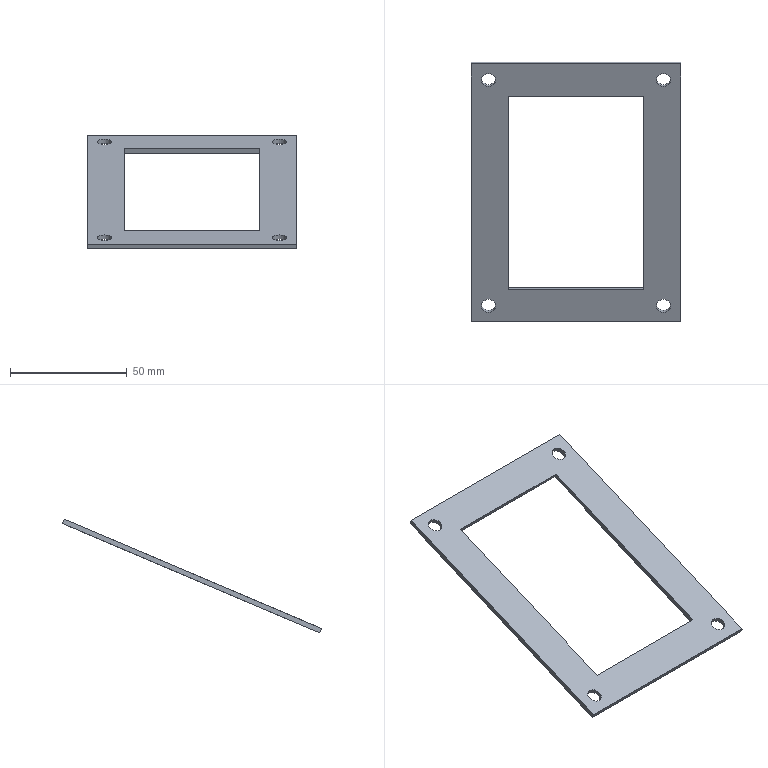Part | NX | features SIMPLE HOLE 56, DATUM_CSYS 27, HOLE PACKAGE 26, SKETCH 26, EXTRUDE 18, EXTRACT_FACE 16, EXTRACT_DATUM_AXIS 10, BLEND 8, CBORE_HOLE 7, EXTRACT_DATUM_PLANE 6, FSET 6, Instance Feature 5, Mirror Feature 5, DRAFT 4, EXTRACT_STRING 2, OFFSET_REGION 1 | 1 solid | 14 faces | box 90 x 111.242 x 48.729 mm | volume 10934 mm3 | plane 10 | cylinder 4 | commonest cylinder face diameters 6 x4
STEP:
#1=CARTESIAN_POINT('',(-45.,-37.433,105.427));
#2=VERTEX_POINT('',#1);
#3=CARTESIAN_POINT('',(-45.,73.028,152.315));
#4=VERTEX_POINT('',#3);
#5=CARTESIAN_POINT('',(-45.,73.028,152.315));
#6=DIRECTION('',(0.,0.9205,0.3907));
#7=VECTOR('',#6,1000.);
#8=LINE('',#5,#7);
#9=EDGE_CURVE('',#2,#4,#8,.T.);
#10=ORIENTED_EDGE('',*,*,#9,.F.);
#11=CARTESIAN_POINT('',(-45.,-38.214,107.268));
#12=VERTEX_POINT('',#11);
#13=CARTESIAN_POINT('',(-45.,17.27,-23.444));
#14=DIRECTION('',(0.,-0.3907,0.9205));
#15=VECTOR('',#14,1000.);
#16=LINE('',#13,#15);
#17=EDGE_CURVE('',#2,#12,#16,.T.);
#18=ORIENTED_EDGE('',*,*,#17,.T.);
#19=CARTESIAN_POINT('',(-45.,72.246,154.156));
#20=VERTEX_POINT('',#19);
#21=CARTESIAN_POINT('',(-45.,72.246,154.156));
#22=DIRECTION('',(0.,-0.9205,-0.3907));
#23=VECTOR('',#22,1000.);
#24=LINE('',#21,#23);
#25=EDGE_CURVE('',#20,#12,#24,.T.);
#26=ORIENTED_EDGE('',*,*,#25,.F.);
#27=CARTESIAN_POINT('',(-45.,127.73,23.444));
#28=DIRECTION('',(0.,-0.3907,0.9205));
#29=VECTOR('',#28,1000.);
#30=LINE('',#27,#29);
#31=EDGE_CURVE('',#4,#20,#30,.T.);
#32=ORIENTED_EDGE('',*,*,#31,.F.);
#33=EDGE_LOOP('',(#10,#18,#26,#32));
#34=FACE_BOUND('',#33,.T.);
#35=CARTESIAN_POINT('',(-45.,127.73,23.444));
#36=DIRECTION('',(1.,0.,0.));
#37=DIRECTION('',(0.,0.,-1.));
#38=AXIS2_PLACEMENT_3D('',#35,#36,#37);
#39=PLANE('',#38);
#40=ADVANCED_FACE('',(#34),#39,.F.);
#41=CARTESIAN_POINT('',(45.,73.028,152.315));
#42=VERTEX_POINT('',#41);
#43=CARTESIAN_POINT('',(45.,-37.433,105.427));
#44=VERTEX_POINT('',#43);
#45=CARTESIAN_POINT('',(45.,73.028,152.315));
#46=DIRECTION('',(0.,-0.9205,-0.3907));
#47=VECTOR('',#46,1000.);
#48=LINE('',#45,#47);
#49=EDGE_CURVE('',#42,#44,#48,.T.);
#50=ORIENTED_EDGE('',*,*,#49,.F.);
#51=CARTESIAN_POINT('',(45.,72.246,154.156));
#52=VERTEX_POINT('',#51);
#53=CARTESIAN_POINT('',(45.,73.028,152.315));
#54=DIRECTION('',(0.,0.3907,-0.9205));
#55=VECTOR('',#54,1000.);
#56=LINE('',#53,#55);
#57=EDGE_CURVE('',#52,#42,#56,.T.);
#58=ORIENTED_EDGE('',*,*,#57,.F.);
#59=CARTESIAN_POINT('',(45.,-38.214,107.268));
#60=VERTEX_POINT('',#59);
#61=CARTESIAN_POINT('',(45.,72.246,154.156));
#62=DIRECTION('',(0.,-0.9205,-0.3907));
#63=VECTOR('',#62,1000.);
#64=LINE('',#61,#63);
#65=EDGE_CURVE('',#52,#60,#64,.T.);
#66=ORIENTED_EDGE('',*,*,#65,.T.);
#67=CARTESIAN_POINT('',(45.,-37.433,105.427));
#68=DIRECTION('',(0.,0.3907,-0.9205));
#69=VECTOR('',#68,1000.);
#70=LINE('',#67,#69);
#71=EDGE_CURVE('',#60,#44,#70,.T.);
#72=ORIENTED_EDGE('',*,*,#71,.T.);
#73=EDGE_LOOP('',(#50,#58,#66,#72));
#74=FACE_BOUND('',#73,.T.);
#75=CARTESIAN_POINT('',(45.,73.028,152.315));
#76=DIRECTION('',(-1.,0.,0.));
#77=DIRECTION('',(0.,0.,1.));
#78=AXIS2_PLACEMENT_3D('',#75,#76,#77);
#79=PLANE('',#78);
#80=ADVANCED_FACE('',(#74),#79,.F.);
#81=ORIENTED_EDGE('',*,*,#57,.T.);
#82=CARTESIAN_POINT('',(0.,73.028,152.315));
#83=DIRECTION('',(-1.,0.,0.));
#84=VECTOR('',#83,1000.);
#85=LINE('',#82,#84);
#86=EDGE_CURVE('',#42,#4,#85,.T.);
#87=ORIENTED_EDGE('',*,*,#86,.T.);
#88=ORIENTED_EDGE('',*,*,#31,.T.);
#89=CARTESIAN_POINT('',(-45.,72.246,154.156));
#90=DIRECTION('',(1.,0.,0.));
#91=VECTOR('',#90,1000.);
#92=LINE('',#89,#91);
#93=EDGE_CURVE('',#20,#52,#92,.T.);
#94=ORIENTED_EDGE('',*,*,#93,.T.);
#95=EDGE_LOOP('',(#81,#87,#88,#94));
#96=FACE_BOUND('',#95,.T.);
#97=CARTESIAN_POINT('',(0.,116.662,49.52));
#98=DIRECTION('',(0.,0.9205,0.3907));
#99=DIRECTION('',(0.,-0.3907,0.9205));
#100=AXIS2_PLACEMENT_3D('',#97,#98,#99);
#101=PLANE('',#100);
#102=ADVANCED_FACE('',(#96),#101,.T.);
#103=CARTESIAN_POINT('',(0.,-37.433,105.427));
#104=DIRECTION('',(-1.,0.,0.));
#105=VECTOR('',#104,1000.);
#106=LINE('',#103,#105);
#107=EDGE_CURVE('',#44,#2,#106,.T.);
#108=ORIENTED_EDGE('',*,*,#107,.F.);
#109=ORIENTED_EDGE('',*,*,#71,.F.);
#110=CARTESIAN_POINT('',(-45.,-38.214,107.268));
#111=DIRECTION('',(1.,0.,0.));
#112=VECTOR('',#111,1000.);
#113=LINE('',#110,#112);
#114=EDGE_CURVE('',#12,#60,#113,.T.);
#115=ORIENTED_EDGE('',*,*,#114,.F.);
#116=ORIENTED_EDGE('',*,*,#17,.F.);
#117=EDGE_LOOP('',(#108,#109,#115,#116));
#118=FACE_BOUND('',#117,.T.);
#119=CARTESIAN_POINT('',(0.,6.201,2.632));
#120=DIRECTION('',(0.,0.9205,0.3907));
#121=DIRECTION('',(0.,-0.3907,0.9205));
#122=AXIS2_PLACEMENT_3D('',#119,#120,#121);
#123=PLANE('',#122);
#124=ADVANCED_FACE('',(#118),#123,.F.);
#125=CARTESIAN_POINT('',(-29.,-24.407,113.129));
#126=VERTEX_POINT('',#125);
#127=CARTESIAN_POINT('',(-29.,-23.625,111.288));
#128=VERTEX_POINT('',#127);
#129=CARTESIAN_POINT('',(-29.,-0.1812,56.057));
#130=DIRECTION('',(0.,-0.3907,0.9205));
#131=VECTOR('',#130,1000.);
#132=LINE('',#129,#131);
#133=EDGE_CURVE('',#126,#128,#132,.F.);
#134=ORIENTED_EDGE('',*,*,#133,.T.);
#135=CARTESIAN_POINT('',(-29.,59.22,146.454));
#136=VERTEX_POINT('',#135);
#137=CARTESIAN_POINT('',(-29.,59.22,146.454));
#138=DIRECTION('',(0.,0.9205,0.3907));
#139=VECTOR('',#138,1000.);
#140=LINE('',#137,#139);
#141=EDGE_CURVE('',#128,#136,#140,.T.);
#142=ORIENTED_EDGE('',*,*,#141,.T.);
#143=CARTESIAN_POINT('',(-29.,58.439,148.295));
#144=VERTEX_POINT('',#143);
#145=CARTESIAN_POINT('',(-29.,82.664,91.223));
#146=DIRECTION('',(0.,-0.3907,0.9205));
#147=VECTOR('',#146,1000.);
#148=LINE('',#145,#147);
#149=EDGE_CURVE('',#144,#136,#148,.F.);
#150=ORIENTED_EDGE('',*,*,#149,.F.);
#151=CARTESIAN_POINT('',(-29.,72.246,154.156));
#152=DIRECTION('',(0.,-0.9205,-0.3907));
#153=VECTOR('',#152,1000.);
#154=LINE('',#151,#153);
#155=EDGE_CURVE('',#144,#126,#154,.T.);
#156=ORIENTED_EDGE('',*,*,#155,.T.);
#157=EDGE_LOOP('',(#134,#142,#150,#156));
#158=FACE_BOUND('',#157,.T.);
#159=CARTESIAN_POINT('',(-29.,82.664,91.223));
#160=DIRECTION('',(1.,0.,0.));
#161=DIRECTION('',(0.,0.,-1.));
#162=AXIS2_PLACEMENT_3D('',#159,#160,#161);
#163=PLANE('',#162);
#164=ADVANCED_FACE('',(#158),#163,.T.);
#165=CARTESIAN_POINT('',(29.,59.22,146.454));
#166=VERTEX_POINT('',#165);
#167=CARTESIAN_POINT('',(29.,58.439,148.295));
#168=VERTEX_POINT('',#167);
#169=CARTESIAN_POINT('',(29.,57.657,150.136));
#170=DIRECTION('',(0.,0.3907,-0.9205));
#171=VECTOR('',#170,1000.);
#172=LINE('',#169,#171);
#173=EDGE_CURVE('',#166,#168,#172,.F.);
#174=ORIENTED_EDGE('',*,*,#173,.F.);
#175=CARTESIAN_POINT('',(29.,-23.625,111.288));
#176=VERTEX_POINT('',#175);
#177=CARTESIAN_POINT('',(29.,59.22,146.454));
#178=DIRECTION('',(0.,-0.9205,-0.3907));
#179=VECTOR('',#178,1000.);
#180=LINE('',#177,#179);
#181=EDGE_CURVE('',#166,#176,#180,.T.);
#182=ORIENTED_EDGE('',*,*,#181,.T.);
#183=CARTESIAN_POINT('',(29.,-24.407,113.129));
#184=VERTEX_POINT('',#183);
#185=CARTESIAN_POINT('',(29.,-25.188,114.97));
#186=DIRECTION('',(0.,0.3907,-0.9205));
#187=VECTOR('',#186,1000.);
#188=LINE('',#185,#187);
#189=EDGE_CURVE('',#176,#184,#188,.F.);
#190=ORIENTED_EDGE('',*,*,#189,.T.);
#191=CARTESIAN_POINT('',(29.,72.246,154.156));
#192=DIRECTION('',(0.,0.9205,0.3907));
#193=VECTOR('',#192,1000.);
#194=LINE('',#191,#193);
#195=EDGE_CURVE('',#184,#168,#194,.T.);
#196=ORIENTED_EDGE('',*,*,#195,.T.);
#197=EDGE_LOOP('',(#174,#182,#190,#196));
#198=FACE_BOUND('',#197,.T.);
#199=CARTESIAN_POINT('',(29.,57.657,150.136));
#200=DIRECTION('',(-1.,0.,0.));
#201=DIRECTION('',(0.,0.,1.));
#202=AXIS2_PLACEMENT_3D('',#199,#200,#201);
#203=PLANE('',#202);
#204=ADVANCED_FACE('',(#198),#203,.T.);
#205=CARTESIAN_POINT('',(0.,59.22,146.454));
#206=DIRECTION('',(-1.,0.,0.));
#207=VECTOR('',#206,1000.);
#208=LINE('',#205,#207);
#209=EDGE_CURVE('',#166,#136,#208,.T.);
#210=ORIENTED_EDGE('',*,*,#209,.F.);
#211=ORIENTED_EDGE('',*,*,#173,.T.);
#212=CARTESIAN_POINT('',(-45.,58.439,148.295));
#213=DIRECTION('',(1.,0.,0.));
#214=VECTOR('',#213,1000.);
#215=LINE('',#212,#214);
#216=EDGE_CURVE('',#144,#168,#215,.T.);
#217=ORIENTED_EDGE('',*,*,#216,.F.);
#218=ORIENTED_EDGE('',*,*,#149,.T.);
#219=EDGE_LOOP('',(#210,#211,#217,#218));
#220=FACE_BOUND('',#219,.T.);
#221=CARTESIAN_POINT('',(0.,102.854,43.659));
#222=DIRECTION('',(0.,0.9205,0.3907));
#223=DIRECTION('',(0.,-0.3907,0.9205));
#224=AXIS2_PLACEMENT_3D('',#221,#222,#223);
#225=PLANE('',#224);
#226=ADVANCED_FACE('',(#220),#225,.F.);
#227=ORIENTED_EDGE('',*,*,#189,.F.);
#228=CARTESIAN_POINT('',(0.,-23.625,111.288));
#229=DIRECTION('',(-1.,0.,0.));
#230=VECTOR('',#229,1000.);
#231=LINE('',#228,#230);
#232=EDGE_CURVE('',#176,#128,#231,.T.);
#233=ORIENTED_EDGE('',*,*,#232,.T.);
#234=ORIENTED_EDGE('',*,*,#133,.F.);
#235=CARTESIAN_POINT('',(-45.,-24.407,113.129));
#236=DIRECTION('',(1.,0.,0.));
#237=VECTOR('',#236,1000.);
#238=LINE('',#235,#237);
#239=EDGE_CURVE('',#126,#184,#238,.T.);
#240=ORIENTED_EDGE('',*,*,#239,.T.);
#241=EDGE_LOOP('',(#227,#233,#234,#240));
#242=FACE_BOUND('',#241,.T.);
#243=CARTESIAN_POINT('',(0.,20.009,8.493));
#244=DIRECTION('',(0.,0.9205,0.3907));
#245=DIRECTION('',(0.,-0.3907,0.9205));
#246=AXIS2_PLACEMENT_3D('',#243,#244,#245);
#247=PLANE('',#246);
#248=ADVANCED_FACE('',(#242),#247,.T.);
#249=CARTESIAN_POINT('',(-37.5,-28.549,111.37));
#250=VERTEX_POINT('',#249);
#251=CARTESIAN_POINT('',(-37.5,-31.31,110.198));
#252=DIRECTION('',(0.,0.3907,-0.9205));
#253=DIRECTION('',(0.,0.9205,0.3907));
#254=AXIS2_PLACEMENT_3D('',#251,#252,#253);
#255=CIRCLE('',#254,3.);
#256=EDGE_CURVE('',#250,#250,#255,.T.);
#257=ORIENTED_EDGE('',*,*,#256,.F.);
#258=EDGE_LOOP('',(#257));
#259=FACE_BOUND('',#258,.T.);
#260=CARTESIAN_POINT('',(-37.5,-27.767,109.529));
#261=VERTEX_POINT('',#260);
#262=CARTESIAN_POINT('',(-37.5,-30.529,108.357));
#263=DIRECTION('',(0.,0.3907,-0.9205));
#264=DIRECTION('',(0.,0.9205,0.3907));
#265=AXIS2_PLACEMENT_3D('',#262,#263,#264);
#266=CIRCLE('',#265,3.);
#267=EDGE_CURVE('',#261,#261,#266,.F.);
#268=ORIENTED_EDGE('',*,*,#267,.F.);
#269=EDGE_LOOP('',(#268));
#270=FACE_BOUND('',#269,.T.);
#271=CARTESIAN_POINT('',(-37.5,-30.529,108.357));
#272=DIRECTION('',(0.,0.3907,-0.9205));
#273=DIRECTION('',(0.,0.9205,0.3907));
#274=AXIS2_PLACEMENT_3D('',#271,#272,#273);
#275=CYLINDRICAL_SURFACE('',#274,3.);
#276=ADVANCED_FACE('',(#259,#270),#275,.F.);
#277=CARTESIAN_POINT('',(-37.5,68.104,152.397));
#278=VERTEX_POINT('',#277);
#279=CARTESIAN_POINT('',(-37.5,65.343,151.225));
#280=DIRECTION('',(0.,0.3907,-0.9205));
#281=DIRECTION('',(0.,0.9205,0.3907));
#282=AXIS2_PLACEMENT_3D('',#279,#280,#281);
#283=CIRCLE('',#282,3.);
#284=EDGE_CURVE('',#278,#278,#283,.T.);
#285=ORIENTED_EDGE('',*,*,#284,.F.);
#286=EDGE_LOOP('',(#285));
#287=FACE_BOUND('',#286,.T.);
#288=CARTESIAN_POINT('',(-37.5,68.886,150.556));
#289=VERTEX_POINT('',#288);
#290=CARTESIAN_POINT('',(-37.5,66.124,149.384));
#291=DIRECTION('',(0.,0.3907,-0.9205));
#292=DIRECTION('',(0.,0.9205,0.3907));
#293=AXIS2_PLACEMENT_3D('',#290,#291,#292);
#294=CIRCLE('',#293,3.);
#295=EDGE_CURVE('',#289,#289,#294,.F.);
#296=ORIENTED_EDGE('',*,*,#295,.F.);
#297=EDGE_LOOP('',(#296));
#298=FACE_BOUND('',#297,.T.);
#299=CARTESIAN_POINT('',(-37.5,66.124,149.384));
#300=DIRECTION('',(0.,0.3907,-0.9205));
#301=DIRECTION('',(0.,0.9205,0.3907));
#302=AXIS2_PLACEMENT_3D('',#299,#300,#301);
#303=CYLINDRICAL_SURFACE('',#302,3.);
#304=ADVANCED_FACE('',(#287,#298),#303,.F.);
#305=CARTESIAN_POINT('',(37.5,-28.549,111.37));
#306=VERTEX_POINT('',#305);
#307=CARTESIAN_POINT('',(37.5,-31.31,110.198));
#308=DIRECTION('',(0.,0.3907,-0.9205));
#309=DIRECTION('',(0.,0.9205,0.3907));
#310=AXIS2_PLACEMENT_3D('',#307,#308,#309);
#311=CIRCLE('',#310,3.);
#312=EDGE_CURVE('',#306,#306,#311,.T.);
#313=ORIENTED_EDGE('',*,*,#312,.F.);
#314=EDGE_LOOP('',(#313));
#315=FACE_BOUND('',#314,.T.);
#316=CARTESIAN_POINT('',(37.5,-27.767,109.529));
#317=VERTEX_POINT('',#316);
#318=CARTESIAN_POINT('',(37.5,-30.529,108.357));
#319=DIRECTION('',(0.,0.3907,-0.9205));
#320=DIRECTION('',(0.,0.9205,0.3907));
#321=AXIS2_PLACEMENT_3D('',#318,#319,#320);
#322=CIRCLE('',#321,3.);
#323=EDGE_CURVE('',#317,#317,#322,.F.);
#324=ORIENTED_EDGE('',*,*,#323,.F.);
#325=EDGE_LOOP('',(#324));
#326=FACE_BOUND('',#325,.T.);
#327=CARTESIAN_POINT('',(37.5,-30.529,108.357));
#328=DIRECTION('',(0.,0.3907,-0.9205));
#329=DIRECTION('',(0.,0.9205,0.3907));
#330=AXIS2_PLACEMENT_3D('',#327,#328,#329);
#331=CYLINDRICAL_SURFACE('',#330,3.);
#332=ADVANCED_FACE('',(#315,#326),#331,.F.);
#333=CARTESIAN_POINT('',(37.5,68.104,152.397));
#334=VERTEX_POINT('',#333);
#335=CARTESIAN_POINT('',(37.5,65.343,151.225));
#336=DIRECTION('',(0.,0.3907,-0.9205));
#337=DIRECTION('',(0.,0.9205,0.3907));
#338=AXIS2_PLACEMENT_3D('',#335,#336,#337);
#339=CIRCLE('',#338,3.);
#340=EDGE_CURVE('',#334,#334,#339,.T.);
#341=ORIENTED_EDGE('',*,*,#340,.F.);
#342=EDGE_LOOP('',(#341));
#343=FACE_BOUND('',#342,.T.);
#344=CARTESIAN_POINT('',(37.5,68.886,150.556));
#345=VERTEX_POINT('',#344);
#346=CARTESIAN_POINT('',(37.5,66.124,149.384));
#347=DIRECTION('',(0.,0.3907,-0.9205));
#348=DIRECTION('',(0.,0.9205,0.3907));
#349=AXIS2_PLACEMENT_3D('',#346,#347,#348);
#350=CIRCLE('',#349,3.);
#351=EDGE_CURVE('',#345,#345,#350,.F.);
#352=ORIENTED_EDGE('',*,*,#351,.F.);
#353=EDGE_LOOP('',(#352));
#354=FACE_BOUND('',#353,.T.);
#355=CARTESIAN_POINT('',(37.5,66.124,149.384));
#356=DIRECTION('',(0.,0.3907,-0.9205));
#357=DIRECTION('',(0.,0.9205,0.3907));
#358=AXIS2_PLACEMENT_3D('',#355,#356,#357);
#359=CYLINDRICAL_SURFACE('',#358,3.);
#360=ADVANCED_FACE('',(#343,#354),#359,.F.);
#361=ORIENTED_EDGE('',*,*,#340,.T.);
#362=EDGE_LOOP('',(#361));
#363=FACE_BOUND('',#362,.T.);
#364=ORIENTED_EDGE('',*,*,#312,.T.);
#365=EDGE_LOOP('',(#364));
#366=FACE_BOUND('',#365,.T.);
#367=ORIENTED_EDGE('',*,*,#284,.T.);
#368=EDGE_LOOP('',(#367));
#369=FACE_BOUND('',#368,.T.);
#370=ORIENTED_EDGE('',*,*,#256,.T.);
#371=EDGE_LOOP('',(#370));
#372=FACE_BOUND('',#371,.T.);
#373=ORIENTED_EDGE('',*,*,#155,.F.);
#374=ORIENTED_EDGE('',*,*,#216,.T.);
#375=ORIENTED_EDGE('',*,*,#195,.F.);
#376=ORIENTED_EDGE('',*,*,#239,.F.);
#377=EDGE_LOOP('',(#373,#374,#375,#376));
#378=FACE_BOUND('',#377,.T.);
#379=ORIENTED_EDGE('',*,*,#114,.T.);
#380=ORIENTED_EDGE('',*,*,#65,.F.);
#381=ORIENTED_EDGE('',*,*,#93,.F.);
#382=ORIENTED_EDGE('',*,*,#25,.T.);
#383=EDGE_LOOP('',(#379,#380,#381,#382));
#384=FACE_BOUND('',#383,.T.);
#385=CARTESIAN_POINT('',(-45.,72.246,154.156));
#386=DIRECTION('',(0.,0.3907,-0.9205));
#387=DIRECTION('',(0.,0.9205,0.3907));
#388=AXIS2_PLACEMENT_3D('',#385,#386,#387);
#389=PLANE('',#388);
#390=ADVANCED_FACE('',(#363,#366,#369,#372,#378,#384),#389,.F.);
#391=ORIENTED_EDGE('',*,*,#49,.T.);
#392=ORIENTED_EDGE('',*,*,#107,.T.);
#393=ORIENTED_EDGE('',*,*,#9,.T.);
#394=ORIENTED_EDGE('',*,*,#86,.F.);
#395=EDGE_LOOP('',(#391,#392,#393,#394));
#396=FACE_BOUND('',#395,.T.);
#397=ORIENTED_EDGE('',*,*,#267,.T.);
#398=EDGE_LOOP('',(#397));
#399=FACE_BOUND('',#398,.T.);
#400=ORIENTED_EDGE('',*,*,#295,.T.);
#401=EDGE_LOOP('',(#400));
#402=FACE_BOUND('',#401,.T.);
#403=ORIENTED_EDGE('',*,*,#323,.T.);
#404=EDGE_LOOP('',(#403));
#405=FACE_BOUND('',#404,.T.);
#406=ORIENTED_EDGE('',*,*,#351,.T.);
#407=EDGE_LOOP('',(#406));
#408=FACE_BOUND('',#407,.T.);
#409=ORIENTED_EDGE('',*,*,#209,.T.);
#410=ORIENTED_EDGE('',*,*,#141,.F.);
#411=ORIENTED_EDGE('',*,*,#232,.F.);
#412=ORIENTED_EDGE('',*,*,#181,.F.);
#413=EDGE_LOOP('',(#409,#410,#411,#412));
#414=FACE_BOUND('',#413,.T.);
#415=CARTESIAN_POINT('',(330.,78.666,154.708));
#416=DIRECTION('',(0.,0.3907,-0.9205));
#417=DIRECTION('',(0.,0.9205,0.3907));
#418=AXIS2_PLACEMENT_3D('',#415,#416,#417);
#419=PLANE('',#418);
#420=ADVANCED_FACE('',(#396,#399,#402,#405,#408,#414),#419,.T.);
#421=CLOSED_SHELL('',(#40,#80,#102,#124,#164,#204,#226,#248,#276,#304,#332,#360,#390,#420));
#422=MANIFOLD_SOLID_BREP('',#421);
#423=(LENGTH_UNIT()NAMED_UNIT(*)SI_UNIT(.MILLI.,.METRE.));
#424=UNCERTAINTY_MEASURE_WITH_UNIT(LENGTH_MEASURE(0.00001),#423,'','');
#425=(NAMED_UNIT(*)PLANE_ANGLE_UNIT()SI_UNIT($,.RADIAN.));
#426=(NAMED_UNIT(*)SI_UNIT($,.STERADIAN.)SOLID_ANGLE_UNIT());
#427=(GEOMETRIC_REPRESENTATION_CONTEXT(3)GLOBAL_UNCERTAINTY_ASSIGNED_CONTEXT((#424))GLOBAL_UNIT_ASSIGNED_CONTEXT((#423,#425,#426))REPRESENTATION_CONTEXT('',''));
#428=ADVANCED_BREP_SHAPE_REPRESENTATION('',(#422),#427);